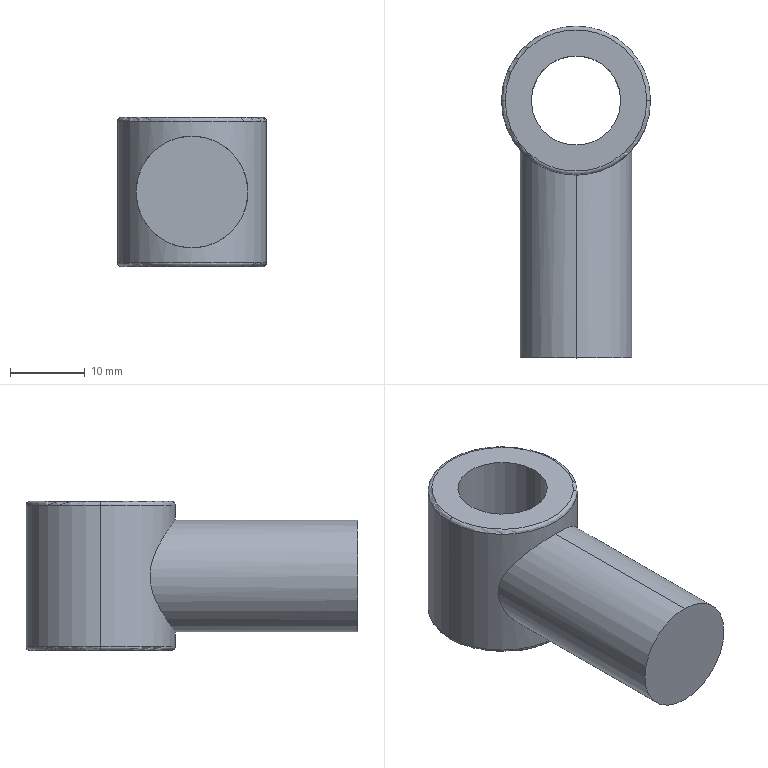Part | STEP file | Hinge | 1 solid | 13 faces | box 20 x 44.5 x 20 mm | volume 8479 mm3 | cylinder 6 | torus 4 | plane 3 | commonest cylinder face diameters 12 x2 15 x2 20 x2
STEP:
#1=CARTESIAN_POINT('',(-10.,104.5,9.5));
#2=VERTEX_POINT('',#1);
#3=CARTESIAN_POINT('',(10.,104.5,9.5));
#4=VERTEX_POINT('',#3);
#5=CARTESIAN_POINT('',(0.,104.5,9.5));
#6=DIRECTION('',(0.,0.,-1.));
#7=DIRECTION('',(1.,0.,0.));
#8=AXIS2_PLACEMENT_3D('',#5,#6,#7);
#9=CIRCLE('',#8,10.);
#10=EDGE_CURVE('',#2,#4,#9,.T.);
#11=ORIENTED_EDGE('',*,*,#10,.F.);
#12=CARTESIAN_POINT('',(-9.5,104.5,10.));
#13=VERTEX_POINT('',#12);
#14=CARTESIAN_POINT('',(-9.5,104.5,9.5));
#15=DIRECTION('',(0.,1.,0.));
#16=DIRECTION('',(-1.,0.,0.));
#17=AXIS2_PLACEMENT_3D('',#14,#15,#16);
#18=CIRCLE('',#17,0.5);
#19=EDGE_CURVE('',#2,#13,#18,.T.);
#20=ORIENTED_EDGE('',*,*,#19,.T.);
#21=CARTESIAN_POINT('',(9.5,104.5,10.));
#22=VERTEX_POINT('',#21);
#23=CARTESIAN_POINT('',(0.,104.5,10.));
#24=DIRECTION('',(0.,0.,1.));
#25=DIRECTION('',(1.,0.,0.));
#26=AXIS2_PLACEMENT_3D('',#23,#24,#25);
#27=CIRCLE('',#26,9.5);
#28=EDGE_CURVE('',#22,#13,#27,.T.);
#29=ORIENTED_EDGE('',*,*,#28,.F.);
#30=CARTESIAN_POINT('',(9.5,104.5,9.5));
#31=DIRECTION('',(0.,-1.,0.));
#32=DIRECTION('',(0.,0.,-1.));
#33=AXIS2_PLACEMENT_3D('',#30,#31,#32);
#34=CIRCLE('',#33,0.5);
#35=EDGE_CURVE('',#4,#22,#34,.T.);
#36=ORIENTED_EDGE('',*,*,#35,.F.);
#37=EDGE_LOOP('',(#11,#20,#29,#36));
#38=FACE_OUTER_BOUND('',#37,.T.);
#39=CARTESIAN_POINT('',(0.,104.5,9.5));
#40=DIRECTION('',(0.,0.,1.));
#41=DIRECTION('',(1.,0.,0.));
#42=AXIS2_PLACEMENT_3D('',#39,#40,#41);
#43=TOROIDAL_SURFACE('',#42,9.5,0.5);
#44=ADVANCED_FACE('',(#38),#43,.T.);
#45=CARTESIAN_POINT('',(-9.5,104.5,-10.));
#46=VERTEX_POINT('',#45);
#47=CARTESIAN_POINT('',(9.5,104.5,-10.));
#48=VERTEX_POINT('',#47);
#49=CARTESIAN_POINT('',(0.,104.5,-10.));
#50=DIRECTION('',(0.,0.,-1.));
#51=DIRECTION('',(1.,0.,0.));
#52=AXIS2_PLACEMENT_3D('',#49,#50,#51);
#53=CIRCLE('',#52,9.5);
#54=EDGE_CURVE('',#46,#48,#53,.T.);
#55=ORIENTED_EDGE('',*,*,#54,.F.);
#56=CARTESIAN_POINT('',(-10.,104.5,-9.5));
#57=VERTEX_POINT('',#56);
#58=CARTESIAN_POINT('',(-9.5,104.5,-9.5));
#59=DIRECTION('',(0.,1.,0.));
#60=DIRECTION('',(-1.,0.,0.));
#61=AXIS2_PLACEMENT_3D('',#58,#59,#60);
#62=CIRCLE('',#61,0.5);
#63=EDGE_CURVE('',#46,#57,#62,.T.);
#64=ORIENTED_EDGE('',*,*,#63,.T.);
#65=CARTESIAN_POINT('',(10.,104.5,-9.5));
#66=VERTEX_POINT('',#65);
#67=CARTESIAN_POINT('',(0.,104.5,-9.5));
#68=DIRECTION('',(0.,0.,1.));
#69=DIRECTION('',(1.,0.,0.));
#70=AXIS2_PLACEMENT_3D('',#67,#68,#69);
#71=CIRCLE('',#70,10.);
#72=EDGE_CURVE('',#66,#57,#71,.T.);
#73=ORIENTED_EDGE('',*,*,#72,.F.);
#74=CARTESIAN_POINT('',(9.5,104.5,-9.5));
#75=DIRECTION('',(0.,-1.,0.));
#76=DIRECTION('',(0.,0.,-1.));
#77=AXIS2_PLACEMENT_3D('',#74,#75,#76);
#78=CIRCLE('',#77,0.5);
#79=EDGE_CURVE('',#48,#66,#78,.T.);
#80=ORIENTED_EDGE('',*,*,#79,.F.);
#81=EDGE_LOOP('',(#55,#64,#73,#80));
#82=FACE_OUTER_BOUND('',#81,.T.);
#83=CARTESIAN_POINT('',(0.,104.5,-9.5));
#84=DIRECTION('',(0.,0.,1.));
#85=DIRECTION('',(1.,0.,0.));
#86=AXIS2_PLACEMENT_3D('',#83,#84,#85);
#87=TOROIDAL_SURFACE('',#86,9.5,0.5);
#88=ADVANCED_FACE('',(#82),#87,.T.);
#89=CARTESIAN_POINT('',(-6.,104.5,-10.));
#90=VERTEX_POINT('',#89);
#91=CARTESIAN_POINT('',(6.,104.5,-10.));
#92=VERTEX_POINT('',#91);
#93=CARTESIAN_POINT('',(0.,104.5,-10.));
#94=DIRECTION('',(0.,0.,1.));
#95=DIRECTION('',(1.,0.,0.));
#96=AXIS2_PLACEMENT_3D('',#93,#94,#95);
#97=CIRCLE('',#96,6.);
#98=EDGE_CURVE('',#90,#92,#97,.T.);
#99=ORIENTED_EDGE('',*,*,#98,.F.);
#100=CARTESIAN_POINT('',(-6.,104.5,10.));
#101=VERTEX_POINT('',#100);
#102=CARTESIAN_POINT('',(-6.,104.5,-10.));
#103=DIRECTION('',(0.,0.,1.));
#104=VECTOR('',#103,1000.);
#105=LINE('',#102,#104);
#106=EDGE_CURVE('',#90,#101,#105,.T.);
#107=ORIENTED_EDGE('',*,*,#106,.T.);
#108=CARTESIAN_POINT('',(6.,104.5,10.));
#109=VERTEX_POINT('',#108);
#110=CARTESIAN_POINT('',(0.,104.5,10.));
#111=DIRECTION('',(0.,0.,1.));
#112=DIRECTION('',(1.,0.,0.));
#113=AXIS2_PLACEMENT_3D('',#110,#111,#112);
#114=CIRCLE('',#113,6.);
#115=EDGE_CURVE('',#101,#109,#114,.T.);
#116=ORIENTED_EDGE('',*,*,#115,.T.);
#117=CARTESIAN_POINT('',(6.,104.5,-10.));
#118=DIRECTION('',(0.,0.,1.));
#119=VECTOR('',#118,1000.);
#120=LINE('',#117,#119);
#121=EDGE_CURVE('',#92,#109,#120,.T.);
#122=ORIENTED_EDGE('',*,*,#121,.F.);
#123=EDGE_LOOP('',(#99,#107,#116,#122));
#124=FACE_OUTER_BOUND('',#123,.T.);
#125=CARTESIAN_POINT('',(0.,104.5,-10.));
#126=DIRECTION('',(0.,0.,1.));
#127=DIRECTION('',(1.,0.,0.));
#128=AXIS2_PLACEMENT_3D('',#125,#126,#127);
#129=CYLINDRICAL_SURFACE('',#128,6.);
#130=ADVANCED_FACE('',(#124),#129,.F.);
#131=ORIENTED_EDGE('',*,*,#10,.T.);
#132=CARTESIAN_POINT('',(10.,104.5,10.));
#133=DIRECTION('',(0.,0.,-1.));
#134=VECTOR('',#133,1000.);
#135=LINE('',#132,#134);
#136=EDGE_CURVE('',#4,#66,#135,.T.);
#137=ORIENTED_EDGE('',*,*,#136,.T.);
#138=ORIENTED_EDGE('',*,*,#72,.T.);
#139=CARTESIAN_POINT('',(-10.,104.5,10.));
#140=DIRECTION('',(0.,0.,-1.));
#141=VECTOR('',#140,1000.);
#142=LINE('',#139,#141);
#143=EDGE_CURVE('',#2,#57,#142,.T.);
#144=ORIENTED_EDGE('',*,*,#143,.F.);
#145=EDGE_LOOP('',(#131,#137,#138,#144));
#146=FACE_OUTER_BOUND('',#145,.T.);
#147=CARTESIAN_POINT('',(0.,104.5,10.));
#148=DIRECTION('',(0.,0.,-1.));
#149=DIRECTION('',(-1.,0.,0.));
#150=AXIS2_PLACEMENT_3D('',#147,#148,#149);
#151=CYLINDRICAL_SURFACE('',#150,10.);
#152=ADVANCED_FACE('',(#146),#151,.T.);
#153=CARTESIAN_POINT('',(0.,70.,-7.5));
#154=VERTEX_POINT('',#153);
#155=CARTESIAN_POINT('',(0.,70.,7.5));
#156=VERTEX_POINT('',#155);
#157=CARTESIAN_POINT('',(0.,70.,0.));
#158=DIRECTION('',(0.,-1.,0.));
#159=DIRECTION('',(0.,0.,-1.));
#160=AXIS2_PLACEMENT_3D('',#157,#158,#159);
#161=CIRCLE('',#160,7.5);
#162=EDGE_CURVE('',#154,#156,#161,.T.);
#163=ORIENTED_EDGE('',*,*,#162,.F.);
#164=CARTESIAN_POINT('',(0.,94.5,-7.5));
#165=VERTEX_POINT('',#164);
#166=CARTESIAN_POINT('',(0.,63.204,-7.5));
#167=DIRECTION('',(0.,1.,0.));
#168=VECTOR('',#167,1000.);
#169=LINE('',#166,#168);
#170=EDGE_CURVE('',#154,#165,#169,.T.);
#171=ORIENTED_EDGE('',*,*,#170,.T.);
#172=CARTESIAN_POINT('',(0.,94.5,7.5));
#173=VERTEX_POINT('',#172);
#174=CARTESIAN_POINT('',(0.,94.5,-7.5));
#175=CARTESIAN_POINT('',(0.2563,94.5,-7.5));
#176=CARTESIAN_POINT('',(0.516,94.51,-7.487));
#177=CARTESIAN_POINT('',(1.029,94.55,-7.434));
#178=CARTESIAN_POINT('',(1.282,94.579,-7.394));
#179=CARTESIAN_POINT('',(1.778,94.656,-7.291));
#180=CARTESIAN_POINT('',(2.022,94.703,-7.227));
#181=CARTESIAN_POINT('',(2.502,94.815,-7.075));
#182=CARTESIAN_POINT('',(2.739,94.879,-6.986));
#183=CARTESIAN_POINT('',(3.422,95.092,-6.692));
#184=CARTESIAN_POINT('',(3.847,95.259,-6.457));
#185=CARTESIAN_POINT('',(4.643,95.632,-5.91));
#186=CARTESIAN_POINT('',(5.006,95.835,-5.604));
#187=CARTESIAN_POINT('',(5.501,96.147,-5.103));
#188=CARTESIAN_POINT('',(5.658,96.252,-4.929));
#189=CARTESIAN_POINT('',(5.955,96.465,-4.565));
#190=CARTESIAN_POINT('',(6.097,96.572,-4.375));
#191=CARTESIAN_POINT('',(6.489,96.884,-3.789));
#192=CARTESIAN_POINT('',(6.714,97.085,-3.376));
#193=CARTESIAN_POINT('',(6.995,97.353,-2.715));
#194=CARTESIAN_POINT('',(7.08,97.437,-2.487));
#195=CARTESIAN_POINT('',(7.228,97.589,-2.015));
#196=CARTESIAN_POINT('',(7.292,97.657,-1.772));
#197=CARTESIAN_POINT('',(7.394,97.767,-1.279));
#198=CARTESIAN_POINT('',(7.434,97.811,-1.029));
#199=CARTESIAN_POINT('',(7.486,97.87,-0.5188));
#200=CARTESIAN_POINT('',(7.5,97.886,-0.2571));
#201=CARTESIAN_POINT('',(7.5,97.886,0.2591));
#202=CARTESIAN_POINT('',(7.487,97.87,0.515));
#203=CARTESIAN_POINT('',(7.434,97.812,1.023));
#204=CARTESIAN_POINT('',(7.395,97.768,1.276));
#205=CARTESIAN_POINT('',(7.24,97.601,2.021));
#206=CARTESIAN_POINT('',(7.092,97.445,2.487));
#207=CARTESIAN_POINT('',(6.809,97.175,3.153));
#208=CARTESIAN_POINT('',(6.704,97.079,3.371));
#209=CARTESIAN_POINT('',(6.476,96.879,3.79));
#210=CARTESIAN_POINT('',(6.354,96.776,3.992));
#211=CARTESIAN_POINT('',(5.962,96.464,4.575));
#212=CARTESIAN_POINT('',(5.667,96.252,4.935));
#213=CARTESIAN_POINT('',(5.171,95.938,5.438));
#214=CARTESIAN_POINT('',(4.995,95.834,5.6));
#215=CARTESIAN_POINT('',(4.63,95.634,5.905));
#216=CARTESIAN_POINT('',(4.441,95.538,6.048));
#217=CARTESIAN_POINT('',(3.852,95.262,6.453));
#218=CARTESIAN_POINT('',(3.431,95.095,6.688));
#219=CARTESIAN_POINT('',(2.748,94.882,6.983));
#220=CARTESIAN_POINT('',(2.511,94.817,7.072));
#221=CARTESIAN_POINT('',(2.03,94.705,7.224));
#222=CARTESIAN_POINT('',(1.786,94.658,7.289));
#223=CARTESIAN_POINT('',(1.289,94.58,7.393));
#224=CARTESIAN_POINT('',(1.036,94.55,7.433));
#225=CARTESIAN_POINT('',(0.5214,94.51,7.486));
#226=CARTESIAN_POINT('',(0.2596,94.5,7.5));
#227=CARTESIAN_POINT('',(0.,94.5,7.5));
#228=B_SPLINE_CURVE_WITH_KNOTS('',3,(#174,#175,#176,#177,#178,#179,#180,#181,#182,#183,#184,#185,#186,#187,#188,#189,#190,#191,#192,#193,#194,#195,#196,#197,#198,#199,#200,#201,#202,#203,#204,#205,#206,#207,#208,#209,#210,#211,#212,#213,#214,#215,#216,#217,#218,#219,#220,#221,#222,#223,#224,#225,#226,#227),.UNSPECIFIED.,.F.,.F.,(4,2,2,2,2,2,2,2,2,2,2,2,2,2,2,2,2,2,2,2,2,2,2,2,2,2,4),(0.02456,0.02533,0.0261,0.02686,0.02763,0.02916,0.03069,0.03146,0.03222,0.03376,0.03452,0.03529,0.03605,0.03682,0.03759,0.03835,0.03989,0.04065,0.04142,0.04295,0.04372,0.04448,0.04601,0.04678,0.04755,0.04831,0.04908),.UNSPECIFIED.);
#229=EDGE_CURVE('',#165,#173,#228,.T.);
#230=ORIENTED_EDGE('',*,*,#229,.T.);
#231=CARTESIAN_POINT('',(0.,63.204,7.5));
#232=DIRECTION('',(0.,1.,0.));
#233=VECTOR('',#232,1000.);
#234=LINE('',#231,#233);
#235=EDGE_CURVE('',#156,#173,#234,.T.);
#236=ORIENTED_EDGE('',*,*,#235,.F.);
#237=EDGE_LOOP('',(#163,#171,#230,#236));
#238=FACE_OUTER_BOUND('',#237,.T.);
#239=CARTESIAN_POINT('',(0.,63.204,0.));
#240=DIRECTION('',(0.,1.,0.));
#241=DIRECTION('',(0.,0.,1.));
#242=AXIS2_PLACEMENT_3D('',#239,#240,#241);
#243=CYLINDRICAL_SURFACE('',#242,7.5);
#244=ADVANCED_FACE('',(#238),#243,.T.);
#245=ORIENTED_EDGE('',*,*,#170,.F.);
#246=CARTESIAN_POINT('',(0.,70.,0.));
#247=DIRECTION('',(0.,-1.,0.));
#248=DIRECTION('',(0.,0.,-1.));
#249=AXIS2_PLACEMENT_3D('',#246,#247,#248);
#250=CIRCLE('',#249,7.5);
#251=EDGE_CURVE('',#156,#154,#250,.T.);
#252=ORIENTED_EDGE('',*,*,#251,.F.);
#253=ORIENTED_EDGE('',*,*,#235,.T.);
#254=CARTESIAN_POINT('',(0.,94.5,7.5));
#255=CARTESIAN_POINT('',(-0.5202,94.5,7.5));
#256=CARTESIAN_POINT('',(-1.028,94.54,7.446));
#257=CARTESIAN_POINT('',(-1.773,94.655,7.292));
#258=CARTESIAN_POINT('',(-2.02,94.703,7.227));
#259=CARTESIAN_POINT('',(-2.503,94.815,7.075));
#260=CARTESIAN_POINT('',(-2.736,94.879,6.987));
#261=CARTESIAN_POINT('',(-3.19,95.019,6.792));
#262=CARTESIAN_POINT('',(-3.41,95.097,6.685));
#263=CARTESIAN_POINT('',(-3.837,95.262,6.449));
#264=CARTESIAN_POINT('',(-4.044,95.352,6.321));
#265=CARTESIAN_POINT('',(-4.641,95.631,5.911));
#266=CARTESIAN_POINT('',(-5.003,95.833,5.607));
#267=CARTESIAN_POINT('',(-5.665,96.25,4.938));
#268=CARTESIAN_POINT('',(-5.965,96.467,4.571));
#269=CARTESIAN_POINT('',(-6.487,96.882,3.793));
#270=CARTESIAN_POINT('',(-6.713,97.083,3.38));
#271=CARTESIAN_POINT('',(-6.996,97.354,2.714));
#272=CARTESIAN_POINT('',(-7.082,97.439,2.482));
#273=CARTESIAN_POINT('',(-7.23,97.59,2.011));
#274=CARTESIAN_POINT('',(-7.292,97.657,1.771));
#275=CARTESIAN_POINT('',(-7.394,97.767,1.279));
#276=CARTESIAN_POINT('',(-7.434,97.811,1.027));
#277=CARTESIAN_POINT('',(-7.487,97.871,0.5128));
#278=CARTESIAN_POINT('',(-7.5,97.886,0.2562));
#279=CARTESIAN_POINT('',(-7.5,97.886,-0.256));
#280=CARTESIAN_POINT('',(-7.487,97.871,-0.5115));
#281=CARTESIAN_POINT('',(-7.435,97.812,-1.021));
#282=CARTESIAN_POINT('',(-7.395,97.768,-1.277));
#283=CARTESIAN_POINT('',(-7.292,97.657,-1.771));
#284=CARTESIAN_POINT('',(-7.229,97.59,-2.011));
#285=CARTESIAN_POINT('',(-7.082,97.439,-2.482));
#286=CARTESIAN_POINT('',(-6.996,97.353,-2.714));
#287=CARTESIAN_POINT('',(-6.712,97.082,-3.382));
#288=CARTESIAN_POINT('',(-6.485,96.881,-3.796));
#289=CARTESIAN_POINT('',(-5.962,96.465,-4.574));
#290=CARTESIAN_POINT('',(-5.661,96.247,-4.942));
#291=CARTESIAN_POINT('',(-5.,95.831,-5.61));
#292=CARTESIAN_POINT('',(-4.639,95.63,-5.913));
#293=CARTESIAN_POINT('',(-3.848,95.26,-6.455));
#294=CARTESIAN_POINT('',(-3.415,95.089,-6.696));
#295=CARTESIAN_POINT('',(-2.734,94.878,-6.988));
#296=CARTESIAN_POINT('',(-2.501,94.815,-7.075));
#297=CARTESIAN_POINT('',(-2.022,94.704,-7.227));
#298=CARTESIAN_POINT('',(-1.775,94.655,-7.292));
#299=CARTESIAN_POINT('',(-1.022,94.539,-7.448));
#300=CARTESIAN_POINT('',(-0.5138,94.5,-7.5));
#301=CARTESIAN_POINT('',(0.,94.5,-7.5));
#302=B_SPLINE_CURVE_WITH_KNOTS('',3,(#254,#255,#256,#257,#258,#259,#260,#261,#262,#263,#264,#265,#266,#267,#268,#269,#270,#271,#272,#273,#274,#275,#276,#277,#278,#279,#280,#281,#282,#283,#284,#285,#286,#287,#288,#289,#290,#291,#292,#293,#294,#295,#296,#297,#298,#299,#300,#301),.UNSPECIFIED.,.F.,.F.,(4,2,2,2,2,2,2,2,2,2,2,2,2,2,2,2,2,2,2,2,2,2,2,4),(0.,0.001535,0.002303,0.003071,0.003838,0.004606,0.006141,0.007676,0.009212,0.009979,0.01075,0.01151,0.01228,0.01305,0.01382,0.01459,0.01535,0.01689,0.01842,0.01996,0.02149,0.02226,0.02303,0.02456),.UNSPECIFIED.);
#303=EDGE_CURVE('',#173,#165,#302,.T.);
#304=ORIENTED_EDGE('',*,*,#303,.T.);
#305=EDGE_LOOP('',(#245,#252,#253,#304));
#306=FACE_OUTER_BOUND('',#305,.T.);
#307=CARTESIAN_POINT('',(0.,63.204,0.));
#308=DIRECTION('',(0.,1.,0.));
#309=DIRECTION('',(0.,0.,1.));
#310=AXIS2_PLACEMENT_3D('',#307,#308,#309);
#311=CYLINDRICAL_SURFACE('',#310,7.5);
#312=ADVANCED_FACE('',(#306),#311,.T.);
#313=ORIENTED_EDGE('',*,*,#136,.F.);
#314=CARTESIAN_POINT('',(0.,104.5,9.5));
#315=DIRECTION('',(0.,0.,-1.));
#316=DIRECTION('',(1.,0.,0.));
#317=AXIS2_PLACEMENT_3D('',#314,#315,#316);
#318=CIRCLE('',#317,10.);
#319=EDGE_CURVE('',#4,#2,#318,.T.);
#320=ORIENTED_EDGE('',*,*,#319,.T.);
#321=ORIENTED_EDGE('',*,*,#143,.T.);
#322=CARTESIAN_POINT('',(0.,104.5,-9.5));
#323=DIRECTION('',(0.,0.,1.));
#324=DIRECTION('',(1.,0.,0.));
#325=AXIS2_PLACEMENT_3D('',#322,#323,#324);
#326=CIRCLE('',#325,10.);
#327=EDGE_CURVE('',#57,#66,#326,.T.);
#328=ORIENTED_EDGE('',*,*,#327,.T.);
#329=EDGE_LOOP('',(#313,#320,#321,#328));
#330=FACE_OUTER_BOUND('',#329,.T.);
#331=ORIENTED_EDGE('',*,*,#303,.F.);
#332=ORIENTED_EDGE('',*,*,#229,.F.);
#333=EDGE_LOOP('',(#331,#332));
#334=FACE_BOUND('',#333,.T.);
#335=CARTESIAN_POINT('',(0.,104.5,10.));
#336=DIRECTION('',(0.,0.,-1.));
#337=DIRECTION('',(-1.,0.,0.));
#338=AXIS2_PLACEMENT_3D('',#335,#336,#337);
#339=CYLINDRICAL_SURFACE('',#338,10.);
#340=ADVANCED_FACE('',(#330,#334),#339,.T.);
#341=ORIENTED_EDGE('',*,*,#28,.T.);
#342=CARTESIAN_POINT('',(0.,104.5,10.));
#343=DIRECTION('',(0.,0.,1.));
#344=DIRECTION('',(1.,0.,0.));
#345=AXIS2_PLACEMENT_3D('',#342,#343,#344);
#346=CIRCLE('',#345,9.5);
#347=EDGE_CURVE('',#13,#22,#346,.T.);
#348=ORIENTED_EDGE('',*,*,#347,.T.);
#349=EDGE_LOOP('',(#341,#348));
#350=FACE_OUTER_BOUND('',#349,.T.);
#351=CARTESIAN_POINT('',(0.,104.5,10.));
#352=DIRECTION('',(0.,0.,1.));
#353=DIRECTION('',(1.,0.,0.));
#354=AXIS2_PLACEMENT_3D('',#351,#352,#353);
#355=CIRCLE('',#354,6.);
#356=EDGE_CURVE('',#109,#101,#355,.T.);
#357=ORIENTED_EDGE('',*,*,#356,.F.);
#358=ORIENTED_EDGE('',*,*,#115,.F.);
#359=EDGE_LOOP('',(#357,#358));
#360=FACE_BOUND('',#359,.T.);
#361=CARTESIAN_POINT('',(0.,104.5,10.));
#362=DIRECTION('',(0.,0.,1.));
#363=DIRECTION('',(1.,0.,0.));
#364=AXIS2_PLACEMENT_3D('',#361,#362,#363);
#365=PLANE('',#364);
#366=ADVANCED_FACE('',(#350,#360),#365,.T.);
#367=CARTESIAN_POINT('',(0.,104.5,-10.));
#368=DIRECTION('',(0.,0.,-1.));
#369=DIRECTION('',(1.,0.,0.));
#370=AXIS2_PLACEMENT_3D('',#367,#368,#369);
#371=CIRCLE('',#370,9.5);
#372=EDGE_CURVE('',#48,#46,#371,.T.);
#373=ORIENTED_EDGE('',*,*,#372,.T.);
#374=ORIENTED_EDGE('',*,*,#54,.T.);
#375=EDGE_LOOP('',(#373,#374));
#376=FACE_OUTER_BOUND('',#375,.T.);
#377=CARTESIAN_POINT('',(0.,104.5,-10.));
#378=DIRECTION('',(0.,0.,1.));
#379=DIRECTION('',(1.,0.,0.));
#380=AXIS2_PLACEMENT_3D('',#377,#378,#379);
#381=CIRCLE('',#380,6.);
#382=EDGE_CURVE('',#92,#90,#381,.T.);
#383=ORIENTED_EDGE('',*,*,#382,.T.);
#384=ORIENTED_EDGE('',*,*,#98,.T.);
#385=EDGE_LOOP('',(#383,#384));
#386=FACE_BOUND('',#385,.T.);
#387=CARTESIAN_POINT('',(0.,104.5,-10.));
#388=DIRECTION('',(0.,0.,1.));
#389=DIRECTION('',(1.,0.,0.));
#390=AXIS2_PLACEMENT_3D('',#387,#388,#389);
#391=PLANE('',#390);
#392=ADVANCED_FACE('',(#376,#386),#391,.F.);
#393=ORIENTED_EDGE('',*,*,#106,.F.);
#394=ORIENTED_EDGE('',*,*,#382,.F.);
#395=ORIENTED_EDGE('',*,*,#121,.T.);
#396=ORIENTED_EDGE('',*,*,#356,.T.);
#397=EDGE_LOOP('',(#393,#394,#395,#396));
#398=FACE_OUTER_BOUND('',#397,.T.);
#399=CARTESIAN_POINT('',(0.,104.5,-10.));
#400=DIRECTION('',(0.,0.,1.));
#401=DIRECTION('',(1.,0.,0.));
#402=AXIS2_PLACEMENT_3D('',#399,#400,#401);
#403=CYLINDRICAL_SURFACE('',#402,6.);
#404=ADVANCED_FACE('',(#398),#403,.F.);
#405=ORIENTED_EDGE('',*,*,#63,.F.);
#406=ORIENTED_EDGE('',*,*,#372,.F.);
#407=ORIENTED_EDGE('',*,*,#79,.T.);
#408=ORIENTED_EDGE('',*,*,#327,.F.);
#409=EDGE_LOOP('',(#405,#406,#407,#408));
#410=FACE_OUTER_BOUND('',#409,.T.);
#411=CARTESIAN_POINT('',(0.,104.5,-9.5));
#412=DIRECTION('',(0.,0.,1.));
#413=DIRECTION('',(1.,0.,0.));
#414=AXIS2_PLACEMENT_3D('',#411,#412,#413);
#415=TOROIDAL_SURFACE('',#414,9.5,0.5);
#416=ADVANCED_FACE('',(#410),#415,.T.);
#417=ORIENTED_EDGE('',*,*,#19,.F.);
#418=ORIENTED_EDGE('',*,*,#319,.F.);
#419=ORIENTED_EDGE('',*,*,#35,.T.);
#420=ORIENTED_EDGE('',*,*,#347,.F.);
#421=EDGE_LOOP('',(#417,#418,#419,#420));
#422=FACE_OUTER_BOUND('',#421,.T.);
#423=CARTESIAN_POINT('',(0.,104.5,9.5));
#424=DIRECTION('',(0.,0.,1.));
#425=DIRECTION('',(1.,0.,0.));
#426=AXIS2_PLACEMENT_3D('',#423,#424,#425);
#427=TOROIDAL_SURFACE('',#426,9.5,0.5);
#428=ADVANCED_FACE('',(#422),#427,.T.);
#429=ORIENTED_EDGE('',*,*,#251,.T.);
#430=ORIENTED_EDGE('',*,*,#162,.T.);
#431=EDGE_LOOP('',(#429,#430));
#432=FACE_OUTER_BOUND('',#431,.T.);
#433=CARTESIAN_POINT('',(0.,70.,0.));
#434=DIRECTION('',(0.,-1.,0.));
#435=DIRECTION('',(0.,0.,-1.));
#436=AXIS2_PLACEMENT_3D('',#433,#434,#435);
#437=PLANE('',#436);
#438=ADVANCED_FACE('',(#432),#437,.T.);
#439=CLOSED_SHELL('',(#44,#88,#130,#152,#244,#312,#340,#366,#392,#404,#416,#428,#438));
#440=MANIFOLD_SOLID_BREP('',#439);
#441=CARTESIAN_POINT('',(0.,0.,0.));
#442=DIRECTION('',(0.,0.,1.));
#443=DIRECTION('',(1.,0.,0.));
#444=AXIS2_PLACEMENT_3D('',#441,#442,#443);
#445=(LENGTH_UNIT()NAMED_UNIT(*)SI_UNIT(.MILLI.,.METRE.));
#446=UNCERTAINTY_MEASURE_WITH_UNIT(LENGTH_MEASURE(0.00001),#445,'','');
#447=(NAMED_UNIT(*)PLANE_ANGLE_UNIT()SI_UNIT($,.RADIAN.));
#448=(NAMED_UNIT(*)SI_UNIT($,.STERADIAN.)SOLID_ANGLE_UNIT());
#449=(GEOMETRIC_REPRESENTATION_CONTEXT(3)GLOBAL_UNCERTAINTY_ASSIGNED_CONTEXT((#446))GLOBAL_UNIT_ASSIGNED_CONTEXT((#445,#447,#448))REPRESENTATION_CONTEXT('',''));
#450=ADVANCED_BREP_SHAPE_REPRESENTATION('',(#440,#444),#449);